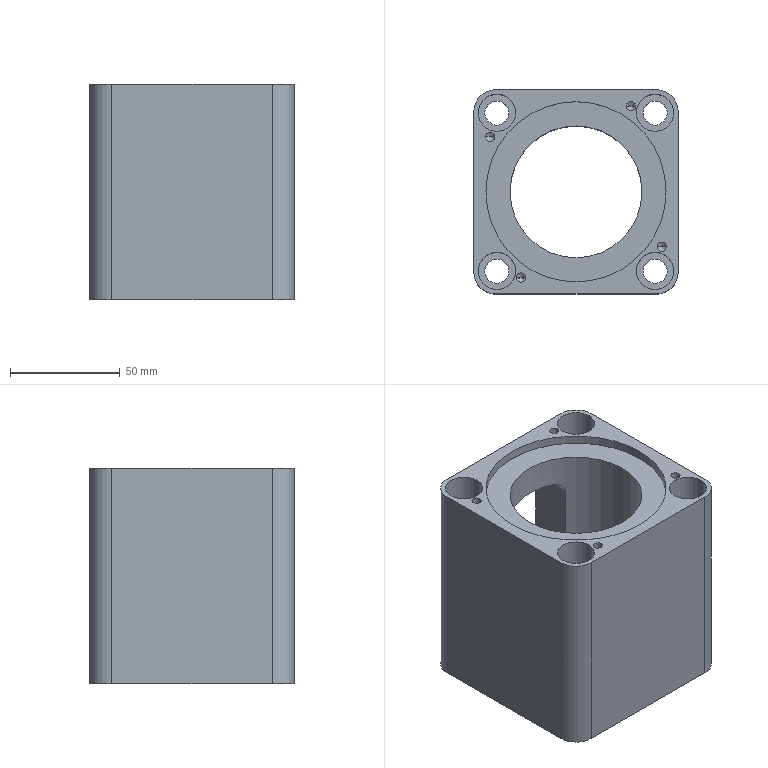Part | SolidWorks | features ICE 5, HoleWzd 4, Fillet 3, CirPattern 1, Extrusion 1 | 1 solid | 86 faces | box 93 x 93 x 98 mm | volume 432719 mm3 | cylinder 50 | plane 20 | cone 16 | commonest cylinder face diameters 2.5 x8 4.2 x8 11 x8 17 x8 6 x4 10 x4